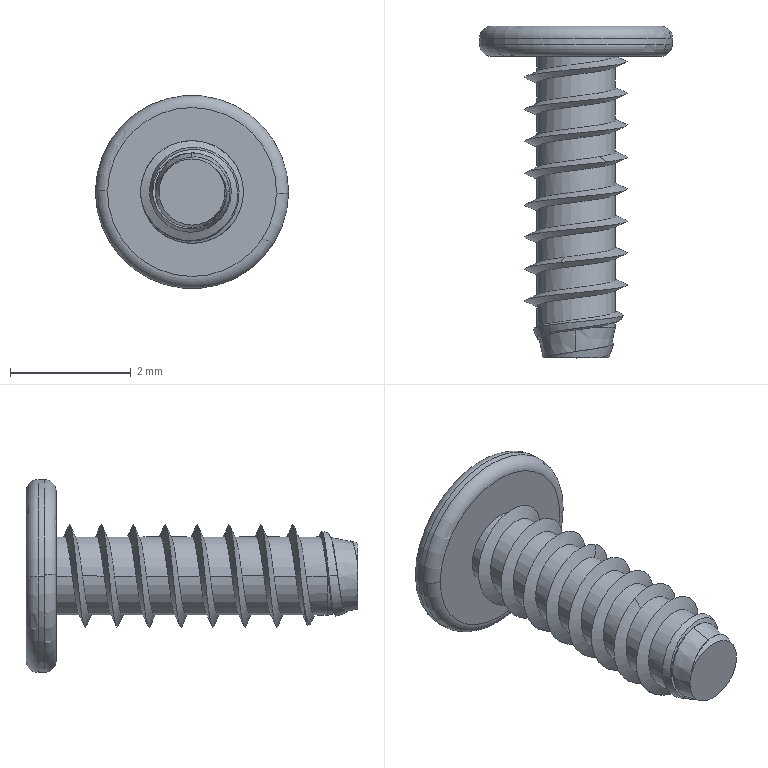Part | SolidWorks | features BaseBody 1 | 1 solid | 59 faces | box 3.2 x 5.5 x 3.2 mm | volume 10.702 mm3 | cylinder 21 | cone 13 | plane 13 | spline 8 | torus 4 | commonest cylinder face diameters 1.3 x19 3.2 x2